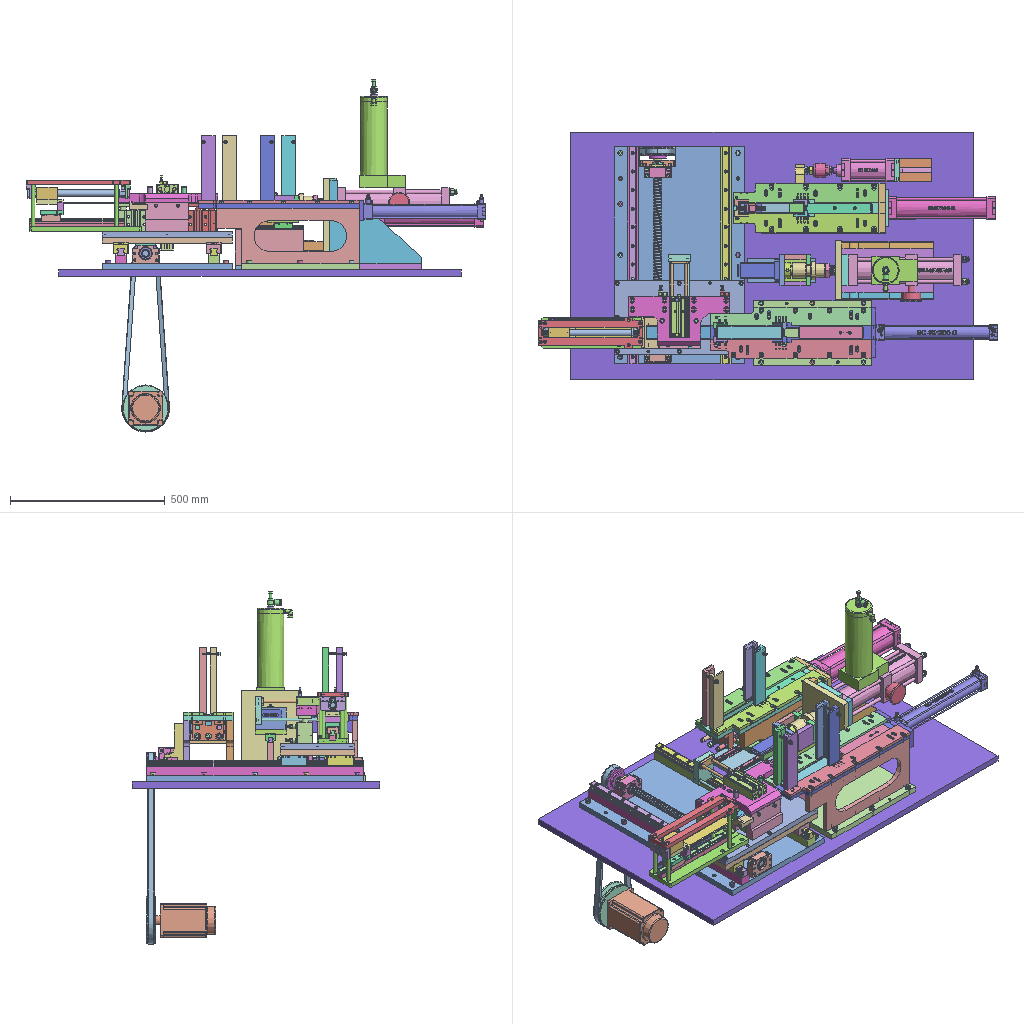Assembly | STEP file | 457 different items | 457 placed | box 1482 x 800 x 1137 mm
Parts list (item | name | quantity | parent item | size | volume), first 304 of 457 items:
1 | Tube feed_id1830_x_t | x1 | in Tube feed_x_t | 460 x 16 x 180 mm | 718962 mm3
2 | Tube feed_id1826_x_t | x1 | in Tube feed_x_t | 13.356 x 6 x 12 mm | 588.844 mm3
3 | Tube feed_id1822_x_t | x1 | in Tube feed_x_t | 13.356 x 6 x 12 mm | 588.844 mm3
4 | Tube feed_id1818_x_t | x1 | in Tube feed_x_t | 10 x 10 x 29.5 mm | 955.443 mm3
5 | Tube feed_id1814_x_t | x1 | in Tube feed_x_t | 10 x 10 x 29.5 mm | 955.443 mm3
6 | Tube feed_id1810_x_t | x1 | in Tube feed_x_t | 10 x 10 x 24.5 mm | 797.459 mm3
7 | Tube feed_id1806_x_t | x1 | in Tube feed_x_t | 10 x 10 x 24.5 mm | 797.459 mm3
8 | Tube feed_id1802_x_t | x1 | in Tube feed_x_t | 10 x 10 x 24.5 mm | 797.459 mm3
9 | Tube feed_id1798_x_t | x1 | in Tube feed_x_t | 10 x 10 x 24.5 mm | 797.459 mm3
10 | Tube feed_id1794_x_t | x1 | in Tube feed_x_t | 10 x 10 x 24.5 mm | 797.459 mm3
11 | Tube feed_id1790_x_t | x1 | in Tube feed_x_t | 8 x 22 x 23.5 mm | 3770 mm3
12 | Tube feed_id1786_x_t | x1 | in Tube feed_x_t | 8 x 22 x 23.5 mm | 3770 mm3
13 | Tube feed_id1782_x_t | x1 | in Tube feed_x_t | 8 x 22 x 23.5 mm | 3770 mm3
14 | Tube feed_id1778_x_t | x1 | in Tube feed_x_t | 8 x 22 x 23.5 mm | 3770 mm3
15 | Tube feed_id1774_x_t | x1 | in Tube feed_x_t | 520 x 160 x 13.5 mm | 851655 mm3
16 | Tube feed_id1770_x_t | x1 | in Tube feed_x_t | 380 x 208.2 x 19.5 mm | 1510900 mm3
17 | Tube feed_id1766_x_t | x1 | in Tube feed_x_t | 380 x 16 x 180 mm | 635735 mm3
18 | Tube feed_id1762_x_t | x1 | in Tube feed_x_t | 8 x 8 x 30 mm | 1469 mm3
19 | Tube feed_id1758_x_t | x1 | in Tube feed_x_t | 8 x 8 x 30 mm | 1469 mm3
20 | Tube feed_id1754_x_t | x1 | in Tube feed_x_t | 8 x 8 x 30 mm | 1469 mm3
21 | Tube feed_id1750_x_t | x1 | in Tube feed_x_t | 8 x 8 x 30 mm | 1469 mm3
22 | Tube feed_id1746_x_t | x1 | in Tube feed_x_t | 10 x 10 x 24.5 mm | 797.459 mm3
23 | Tube feed_id1742_x_t | x1 | in Tube feed_x_t | 13 x 13 x 33 mm | 1945 mm3
24 | Tube feed_id1738_x_t | x1 | in Tube feed_x_t | 8 x 8 x 40 mm | 1972 mm3
25 | Tube feed_id1734_x_t | x1 | in Tube feed_x_t | 8 x 8 x 40 mm | 1972 mm3
26 | Tube feed_id1730_x_t | x1 | in Tube feed_x_t | 16 x 16 x 50 mm | 4036 mm3
27 | Tube feed_id1726_x_t | x1 | in Tube feed_x_t | 16 x 16 x 50 mm | 4036 mm3
28 | Tube feed_id1722_x_t | x1 | in Tube feed_x_t | 16 x 16 x 50 mm | 4036 mm3
29 | Tube feed_id1718_x_t | x1 | in Tube feed_x_t | 16 x 16 x 50 mm | 4397 mm3
30 | Tube feed_id1714_x_t | x1 | in Tube feed_x_t | 16 x 16 x 50 mm | 4397 mm3
31 | Tube feed_id1710_x_t | x1 | in Tube feed_x_t | 16 x 16 x 50 mm | 4397 mm3
32 | Tube feed_id1706_x_t | x1 | in Tube feed_x_t | 8 x 8 x 35 mm | 1721 mm3
33 | Tube feed_id1702_x_t | x1 | in Tube feed_x_t | 8 x 8 x 35 mm | 1721 mm3
34 | Tube feed_id1698_x_t | x1 | in Tube feed_x_t | 8 x 8 x 35 mm | 1721 mm3
35 | Tube feed_id1694_x_t | x1 | in Tube feed_x_t | 8 x 8 x 35 mm | 1721 mm3
36 | Tube feed_id1690_x_t | x1 | in Tube feed_x_t | 13 x 13 x 33 mm | 1974 mm3
37 | Tube feed_id1686_x_t | x1 | in Tube feed_x_t | 13 x 13 x 33 mm | 1974 mm3
38 | Tube feed_id1682_x_t | x1 | in Tube feed_x_t | 13 x 13 x 33 mm | 1974 mm3
39 | Tube feed_id1678_x_t | x1 | in Tube feed_x_t | 13 x 13 x 33 mm | 1974 mm3
40 | Tube feed_id1674_x_t | x1 | in Tube feed_x_t | 13 x 13 x 33 mm | 1974 mm3
41 | Tube feed_id1670_x_t | x1 | in Tube feed_x_t | 13 x 13 x 33 mm | 1974 mm3
42 | Tube feed_id1666_x_t | x1 | in Tube feed_x_t | 13 x 13 x 33 mm | 1974 mm3
43 | Tube feed_id1662_x_t | x1 | in Tube feed_x_t | 13 x 13 x 33 mm | 1974 mm3
44 | Tube feed_id1658_x_t | x1 | in Tube feed_x_t | 13 x 13 x 33 mm | 1945 mm3
45 | Tube feed_id1654_x_t | x1 | in Tube feed_x_t | 13 x 13 x 33 mm | 1945 mm3
46 | Tube feed_id1650_x_t | x1 | in Tube feed_x_t | 13 x 13 x 33 mm | 1945 mm3
47 | Tube feed_id1646_x_t | x1 | in Tube feed_x_t | 13 x 13 x 33 mm | 1945 mm3
48 | Tube feed_id1642_x_t | x1 | in Tube feed_x_t | 13 x 13 x 33 mm | 1945 mm3
49 | Tube feed_id1638_x_t | x1 | in Tube feed_x_t | 13 x 13 x 33 mm | 1945 mm3
50 | Tube feed_id1634_x_t | x1 | in Tube feed_x_t | 13 x 13 x 33 mm | 1945 mm3
51 | Tube feed_id1630_x_t | x1 | in Tube feed_x_t | 13 x 13 x 33 mm | 1945 mm3
52 | Tube feed_id1626_x_t | x1 | in Tube feed_x_t | 16 x 16 x 47 mm | 3975 mm3
53 | Tube feed_id1622_x_t | x1 | in Tube feed_x_t | 16 x 16 x 47 mm | 3975 mm3
54 | Tube feed_id1618_x_t | x1 | in Tube feed_x_t | 16 x 16 x 47 mm | 3975 mm3
55 | Tube feed_id1614_x_t | x1 | in Tube feed_x_t | 16 x 16 x 47 mm | 3975 mm3
56 | Tube feed_id1610_x_t | x1 | in Tube feed_x_t | 16 x 16 x 47 mm | 3975 mm3
57 | Tube feed_id1606_x_t | x1 | in Tube feed_x_t | 10 x 10 x 26 mm | 858.061 mm3
58 | Tube feed_id1602_x_t | x1 | in Tube feed_x_t | 10 x 10 x 26 mm | 858.061 mm3
59 | Tube feed_id1598_x_t | x1 | in Tube feed_x_t | 10 x 10 x 26 mm | 858.061 mm3
60 | Tube feed_id1594_x_t | x1 | in Tube feed_x_t | 10 x 10 x 26 mm | 858.061 mm3
61 | Tube feed_id1590_x_t | x1 | in Tube feed_x_t | 10 x 10 x 26 mm | 858.061 mm3
62 | Tube feed_id1586_x_t | x1 | in Tube feed_x_t | 10 x 10 x 26 mm | 858.061 mm3
63 | Tube feed_id1582_x_t | x1 | in Tube feed_x_t | 10 x 10 x 26 mm | 858.061 mm3
64 | Tube feed_id1578_x_t | x1 | in Tube feed_x_t | 10 x 10 x 26 mm | 858.061 mm3
65 | Tube feed_id1574_x_t | x1 | in Tube feed_x_t | 10 x 10 x 26 mm | 858.061 mm3
66 | Tube feed_id1570_x_t | x1 | in Tube feed_x_t | 23 x 700 x 22 mm | 297908 mm3
67 | Tube feed_id1566_x_t | x1 | in Tube feed_x_t | 12 x 12 x 37 mm | 4054 mm3
68 | Tube feed_id1562_x_t | x1 | in Tube feed_x_t | 12 x 12 x 37 mm | 4054 mm3
69 | Tube feed_id1558_x_t | x1 | in Tube feed_x_t | 12 x 12 x 37 mm | 4054 mm3
70 | Tube feed_id1554_x_t | x1 | in Tube feed_x_t | 12 x 12 x 37 mm | 4054 mm3
71 | Tube feed_id1550_x_t | x1 | in Tube feed_x_t | 16 x 16 x 47 mm | 4055 mm3
72 | Tube feed_id1546_x_t | x1 | in Tube feed_x_t | 16 x 16 x 47 mm | 4055 mm3
73 | Tube feed_id1542_x_t | x1 | in Tube feed_x_t | 16 x 16 x 47 mm | 4055 mm3
74 | Tube feed_id1538_x_t | x1 | in Tube feed_x_t | 16 x 16 x 47 mm | 4055 mm3
75 | Tube feed_id1534_x_t | x1 | in Tube feed_x_t | 16 x 16 x 47 mm | 4055 mm3
76 | Tube feed_id1530_x_t | x1 | in Tube feed_x_t | 10 x 10 x 26 mm | 852.808 mm3
77 | Tube feed_id1526_x_t | x1 | in Tube feed_x_t | 10 x 10 x 26 mm | 852.808 mm3
78 | Tube feed_id1522_x_t | x1 | in Tube feed_x_t | 10 x 10 x 26 mm | 852.808 mm3
79 | Tube feed_id1518_x_t | x1 | in Tube feed_x_t | 10 x 10 x 26 mm | 852.808 mm3
80 | Tube feed_id1514_x_t | x1 | in Tube feed_x_t | 10 x 10 x 26 mm | 852.808 mm3
81 | Tube feed_id1510_x_t | x1 | in Tube feed_x_t | 10 x 10 x 26 mm | 852.808 mm3
82 | Tube feed_id1506_x_t | x1 | in Tube feed_x_t | 10 x 10 x 26 mm | 852.808 mm3
83 | Tube feed_id1502_x_t | x1 | in Tube feed_x_t | 10 x 10 x 26 mm | 852.808 mm3
84 | Tube feed_id1498_x_t | x1 | in Tube feed_x_t | 10 x 10 x 26 mm | 852.808 mm3
85 | Tube feed_id1494_x_t | x1 | in Tube feed_x_t | 10 x 10 x 26 mm | 852.808 mm3
86 | Tube feed_id1490_x_t | x1 | in Tube feed_x_t | 10 x 10 x 26 mm | 852.808 mm3
87 | Tube feed_id1486_x_t | x1 | in Tube feed_x_t | 10 x 10 x 26 mm | 852.808 mm3
88 | Tube feed_id1482_x_t | x1 | in Tube feed_x_t | 23 x 700 x 22 mm | 297908 mm3
89 | Tube feed_id1478_x_t | x1 | in Tube feed_x_t | 10 x 10 x 26 mm | 858.061 mm3
90 | Tube feed_id1474_x_t | x1 | in Tube feed_x_t | 10 x 10 x 26 mm | 858.061 mm3
91 | Tube feed_id1470_x_t | x1 | in Tube feed_x_t | 10 x 10 x 26 mm | 858.061 mm3
92 | Tube feed_id1466_x_t | x1 | in Tube feed_x_t | 35 x 700 x 30 mm | 688178 mm3
93 | Tube feed_id1462_x_t | x1 | in Tube feed_x_t | 35 x 700 x 30 mm | 688178 mm3
94 | Tube feed_id1458_x_t | x1 | in Tube feed_x_t | 13 x 13 x 28 mm | 1716 mm3
95 | Tube feed_id1454_x_t | x1 | in Tube feed_x_t | 13 x 13 x 28 mm | 1716 mm3
96 | Tube feed_id1450_x_t | x1 | in Tube feed_x_t | 13 x 13 x 28 mm | 1716 mm3
97 | Tube feed_id1446_x_t | x1 | in Tube feed_x_t | 13 x 13 x 28 mm | 1716 mm3
98 | Tube feed_id1442_x_t | x1 | in Tube feed_x_t | 13 x 13 x 28 mm | 1716 mm3
99 | Tube feed_id1438_x_t | x1 | in Tube feed_x_t | 13 x 13 x 28 mm | 1716 mm3
100 | Tube feed_id1434_x_t | x1 | in Tube feed_x_t | 13 x 13 x 28 mm | 1716 mm3
101 | Tube feed_id1430_x_t | x1 | in Tube feed_x_t | 13 x 13 x 28 mm | 1716 mm3
102 | Tube feed_id1426_x_t | x1 | in Tube feed_x_t | 13 x 13 x 28 mm | 1716 mm3
103 | Tube feed_id1422_x_t | x1 | in Tube feed_x_t | 13 x 13 x 28 mm | 1716 mm3
104 | Tube feed_id1418_x_t | x1 | in Tube feed_x_t | 13 x 13 x 28 mm | 1716 mm3
105 | Tube feed_id1414_x_t | x1 | in Tube feed_x_t | 13 x 13 x 28 mm | 1716 mm3
106 | Tube feed_id1410_x_t | x1 | in Tube feed_x_t | 8 x 8 x 30 mm | 1469 mm3
107 | Tube feed_id1406_x_t | x1 | in Tube feed_x_t | 8 x 8 x 30 mm | 1469 mm3
108 | Tube feed_id1402_x_t | x1 | in Tube feed_x_t | 8 x 8 x 30 mm | 1469 mm3
109 | Tube feed_id1398_x_t | x1 | in Tube feed_x_t | 8 x 8 x 30 mm | 1469 mm3
110 | Tube feed_id1394_x_t | x1 | in Tube feed_x_t | 8 x 8 x 30 mm | 1469 mm3
111 | Tube feed_id1390_x_t | x1 | in Tube feed_x_t | 8 x 8 x 30 mm | 1469 mm3
112 | 25 lead screw BK_id1386_x_t | x1 | in Tube feed_x_t | 25 x 669.5 x 25 mm | 331480 mm3
113 | BF-20_id1382_x_t | x1 | in Tube feed_x_t | 42 x 12 x 42 mm | 3541 mm3
114 | BF-20_id1378_x_t | x1 | in Tube feed_x_t | 7 x 7 x 7 mm | 179.594 mm3
115 | BF-20_id1374_x_t | x1 | in Tube feed_x_t | - | 179.594 mm3
116 | BF-20_id1370_x_t | x1 | in Tube feed_x_t | - | 179.594 mm3
117 | BF-20_id1366_x_t | x1 | in Tube feed_x_t | 25 x 12 x 25 mm | 2005 mm3
118 | BF-20_id1362_x_t | x1 | in Tube feed_x_t | - | 179.594 mm3
119 | BF-20_id1358_x_t | x1 | in Tube feed_x_t | 7 x 7 x 7 mm | 179.594 mm3
120 | BF-20_id1354_x_t | x1 | in Tube feed_x_t | - | 179.594 mm3
121 | BF-20_id1350_x_t | x1 | in Tube feed_x_t | - | 179.594 mm3
122 | BF-20_id1346_x_t | x1 | in Tube feed_x_t | - | 179.594 mm3
123 | BF-20_id1342_x_t | x1 | in Tube feed_x_t | - | 179.594 mm3
124 | BF-20_id1338_x_t | x1 | in Tube feed_x_t | 88 x 26 x 60 mm | 81051 mm3
125 | BF-20_id1334_x_t | x1 | in Tube feed_x_t | - | 179.594 mm3
126 | BF-20_id1330_x_t | x1 | in Tube feed_x_t | - | 179.594 mm3
127 | BF-20_id1326_x_t | x1 | in Tube feed_x_t | - | 179.594 mm3
128 | BF-20_id1322_x_t | x1 | in Tube feed_x_t | - | 179.594 mm3
129 | BF-20_id1318_x_t | x1 | in Tube feed_x_t | - | 179.594 mm3
130 | BK-20_id1314_x_t | x1 | in Tube feed_x_t | 42 x 12 x 42 mm | 3939 mm3
131 | BK-20_id1310_x_t | x1 | in Tube feed_x_t | 42 x 12 x 42 mm | 4062 mm3
132 | BK-20_id1306_x_t | x1 | in Tube feed_x_t | 6.35 x 6.35 x 6.35 mm | 134.066 mm3
133 | BK-20_id1302_x_t | x1 | in Tube feed_x_t | 6.35 x 6.35 x 6.35 mm | 134.066 mm3
134 | BK-20_id1298_x_t | x1 | in Tube feed_x_t | 6.35 x 6.35 x 6.35 mm | 134.066 mm3
135 | BK-20_id1294_x_t | x1 | in Tube feed_x_t | 6.35 x 6.35 x 6.35 mm | 134.066 mm3
136 | BK-20_id1290_x_t | x1 | in Tube feed_x_t | 6.35 x 6.35 x 6.35 mm | 134.066 mm3
137 | BK-20_id1286_x_t | x1 | in Tube feed_x_t | 6.35 x 6.35 x 6.35 mm | 134.066 mm3
138 | BK-20_id1282_x_t | x1 | in Tube feed_x_t | 6.35 x 6.35 x 6.35 mm | 134.066 mm3
139 | BK-20_id1278_x_t | x1 | in Tube feed_x_t | 6.35 x 6.35 x 6.35 mm | 134.066 mm3
140 | BK-20_id1274_x_t | x1 | in Tube feed_x_t | 6.35 x 6.35 x 6.35 mm | 134.066 mm3
141 | BK-20_id1270_x_t | x1 | in Tube feed_x_t | 6.35 x 6.35 x 6.35 mm | 134.066 mm3
142 | BK-20_id1266_x_t | x1 | in Tube feed_x_t | 6.35 x 6.35 x 6.35 mm | 134.066 mm3
143 | BK-20_id1262_x_t | x1 | in Tube feed_x_t | 6.35 x 6.35 x 6.35 mm | 134.066 mm3
144 | BK-20_id1258_x_t | x1 | in Tube feed_x_t | 6.35 x 6.35 x 6.35 mm | 134.066 mm3
145 | BK-20_id1254_x_t | x1 | in Tube feed_x_t | 27.5 x 12 x 27.5 mm | 2449 mm3
146 | BK-20_id1250_x_t | x1 | in Tube feed_x_t | 27.5 x 12 x 27.5 mm | 2436 mm3
147 | BK-20_id1246_x_t | x1 | in Tube feed_x_t | 25.4 x 8 x 25.4 mm | 1515 mm3
148 | BK-20_id1242_x_t | x1 | in Tube feed_x_t | 6.35 x 6.35 x 6.35 mm | 134.066 mm3
149 | BK-20_id1238_x_t | x1 | in Tube feed_x_t | 6.35 x 6.35 x 6.35 mm | 134.066 mm3
150 | BK-20_id1234_x_t | x1 | in Tube feed_x_t | 38 x 6 x 38 mm | 1518 mm3
151 | BK-20_id1230_x_t | x1 | in Tube feed_x_t | 6.35 x 6.35 x 6.35 mm | 134.066 mm3
152 | BK-20_id1226_x_t | x1 | in Tube feed_x_t | 38 x 6 x 38 mm | 1557 mm3
153 | BK-20_id1222_x_t | x1 | in Tube feed_x_t | 6.35 x 6.35 x 6.35 mm | 134.066 mm3
154 | BK-20_id1218_x_t | x1 | in Tube feed_x_t | 6.35 x 6.35 x 6.35 mm | 134.066 mm3
155 | BK-20_id1214_x_t | x1 | in Tube feed_x_t | 50 x 11.15 x 50 mm | 9475 mm3
156 | BK-20_id1210_x_t | x1 | in Tube feed_x_t | 6.35 x 6.35 x 6.35 mm | 134.066 mm3
157 | BK-20_id1206_x_t | x1 | in Tube feed_x_t | 35 x 11 x 35 mm | 5569 mm3
158 | BK-20_id1202_x_t | x1 | in Tube feed_x_t | 6.35 x 6.35 x 6.35 mm | 134.066 mm3
159 | BK-20_id1198_x_t | x1 | in Tube feed_x_t | 6.35 x 6.35 x 6.35 mm | 134.066 mm3
160 | BK-20_id1194_x_t | x1 | in Tube feed_x_t | 6.35 x 6.35 x 6.35 mm | 134.066 mm3
161 | BK-20_id1190_x_t | x1 | in Tube feed_x_t | 88 x 35 x 60 mm | 106061 mm3
162 | BK-20_id1186_x_t | x1 | in Tube feed_x_t | 6.35 x 6.35 x 6.35 mm | 134.066 mm3
163 | BK-20_id1182_x_t | x1 | in Tube feed_x_t | 6.35 x 6.35 x 6.35 mm | 134.066 mm3
164 | BK-20_id1178_x_t | x1 | in Tube feed_x_t | 6.35 x 6.35 x 6.35 mm | 134.066 mm3
165 | BK-20_id1174_x_t | x1 | in Tube feed_x_t | 6.35 x 6.35 x 6.35 mm | 134.066 mm3
166 | BK-20_id1170_x_t | x1 | in Tube feed_x_t | 25.4 x 8.5 x 25.4 mm | 1588 mm3
167 | Tube feed_id1166_x_t | x1 | in Tube feed_x_t | 420 x 700 x 19.5 mm | 5525930 mm3
168 | Tube feed_id1162_x_t | x1 | in Tube feed_x_t | 13 x 13 x 68 mm | 3686 mm3
169 | Tube feed_id1158_x_t | x1 | in Tube feed_x_t | 13 x 13 x 68 mm | 3686 mm3
170 | Tube feed_id1154_x_t | x1 | in Tube feed_x_t | 13 x 13 x 68 mm | 3686 mm3
171 | Tube feed_id1150_x_t | x1 | in Tube feed_x_t | 13 x 13 x 68 mm | 3686 mm3
172 | Tube feed_id1146_x_t | x1 | in Tube feed_x_t | 13 x 13 x 68 mm | 3686 mm3
173 | Tube feed_id1142_x_t | x1 | in Tube feed_x_t | 13 x 13 x 68 mm | 3686 mm3
174 | Tube feed_id1138_x_t | x1 | in Tube feed_x_t | 8 x 8 x 20 mm | 966.7 mm3
175 | Tube feed_id1134_x_t | x1 | in Tube feed_x_t | 8 x 8 x 20 mm | 966.7 mm3
176 | Tube feed_id1130_x_t | x1 | in Tube feed_x_t | 13 x 13 x 33 mm | 1997 mm3
177 | Tube feed_id1126_x_t | x1 | in Tube feed_x_t | 13 x 13 x 33 mm | 1997 mm3
178 | Tube feed_id1122_x_t | x1 | in Tube feed_x_t | 13 x 13 x 33 mm | 1997 mm3
179 | Tube feed_id1118_x_t | x1 | in Tube feed_x_t | 13 x 13 x 33 mm | 1997 mm3
180 | Tube feed_id1114_x_t | x1 | in Tube feed_x_t | 13 x 13 x 33 mm | 1997 mm3
181 | Tube feed_id1110_x_t | x1 | in Tube feed_x_t | 13 x 13 x 33 mm | 1997 mm3
182 | Tube feed_id1106_x_t | x1 | in Tube feed_x_t | 13 x 13 x 33 mm | 1997 mm3
183 | Tube feed_id1102_x_t | x1 | in Tube feed_x_t | 13 x 13 x 33 mm | 1997 mm3
184 | Tube feed_id1098_x_t | x1 | in Tube feed_x_t | 10 x 10 x 21 mm | 739.091 mm3
185 | Tube feed_id1094_x_t | x1 | in Tube feed_x_t | 10 x 10 x 21 mm | 739.091 mm3
186 | Tube feed_id1090_x_t | x1 | in Tube feed_x_t | 10 x 10 x 21 mm | 739.091 mm3
187 | Tube feed_id1086_x_t | x1 | in Tube feed_x_t | 10 x 10 x 21 mm | 739.091 mm3
188 | Tube feed_id1082_x_t | x1 | in Tube feed_x_t | 10 x 10 x 21 mm | 739.091 mm3
189 | Tube feed_id1078_x_t | x1 | in Tube feed_x_t | 10 x 10 x 21 mm | 739.091 mm3
190 | Tube feed_id1074_x_t | x1 | in Tube feed_x_t | 10 x 10 x 21 mm | 739.091 mm3
191 | Tube feed_id1070_x_t | x1 | in Tube feed_x_t | 10 x 10 x 21 mm | 739.091 mm3
192 | Tube feed_id1066_x_t | x1 | in Tube feed_x_t | 10 x 10 x 21 mm | 739.091 mm3
193 | Tube feed_id1062_x_t | x1 | in Tube feed_x_t | 10 x 10 x 21 mm | 739.091 mm3
194 | Tube feed_id1058_x_t | x1 | in Tube feed_x_t | 10 x 10 x 21 mm | 739.091 mm3
195 | Tube feed_id1054_x_t | x1 | in Tube feed_x_t | 10 x 10 x 21 mm | 739.091 mm3
196 | Tube feed_id1050_x_t | x1 | in Tube feed_x_t | 10 x 10 x 21 mm | 739.091 mm3
197 | Tube feed_id1046_x_t | x1 | in Tube feed_x_t | 10 x 10 x 21 mm | 739.091 mm3
198 | Tube feed_id1042_x_t | x1 | in Tube feed_x_t | 10 x 10 x 21 mm | 739.091 mm3
199 | Tube feed_id1038_x_t | x1 | in Tube feed_x_t | 10 x 10 x 21 mm | 739.091 mm3
200 | Tube feed_id1034_x_t | x1 | in Tube feed_x_t | 10 x 10 x 41 mm | 1187 mm3
201 | Tube feed_id1030_x_t | x1 | in Tube feed_x_t | 10 x 10 x 41 mm | 1187 mm3
202 | Tube feed_id1026_x_t | x1 | in Tube feed_x_t | 10 x 10 x 41 mm | 1187 mm3
203 | Tube feed_id1022_x_t | x1 | in Tube feed_x_t | 10 x 10 x 41 mm | 1187 mm3
204 | Tube feed_id1018_x_t | x1 | in Tube feed_x_t | 66 x 40 x 8 mm | 19888 mm3
205 | Tube feed_id1014_x_t | x1 | in Tube feed_x_t | 420 x 240 x 19.3 mm | 1597092 mm3
206 | SFU2510 nut seat_id1010_x_t | x1 | in Tube feed_x_t | 66 x 85 x 48 mm | 143394 mm3
207 | Tube feed_id1006_x_t | x1 | in Tube feed_x_t | 48 x 95 x 34.5 mm | 104775 mm3
208 | Tube feed_id1002_x_t | x1 | in Tube feed_x_t | 48 x 95 x 34.5 mm | 104775 mm3
209 | Tube feed_id998_x_t | x1 | in Tube feed_x_t | 48 x 95 x 34.5 mm | 104775 mm3
210 | Tube feed_id994_x_t | x1 | in Tube feed_x_t | 48 x 95 x 34.5 mm | 104775 mm3
211 | Tube feed_id990_x_t | x1 | in Tube feed_x_t | 10 x 56 x 10 mm | 1498 mm3
212 | Tube feed_id986_x_t | x1 | in Tube feed_x_t | 10 x 56 x 10 mm | 1498 mm3
213 | Tube feed_id982_x_t | x1 | in Tube feed_x_t | 8 x 19.5 x 8 mm | 422.965 mm3
214 | Tube feed_id978_x_t | x1 | in Tube feed_x_t | 8 x 19.5 x 8 mm | 422.965 mm3
215 | Tube feed_id974_x_t | x1 | in Tube feed_x_t | 8 x 19.5 x 8 mm | 422.965 mm3
216 | Tube feed_id970_x_t | x1 | in Tube feed_x_t | 8 x 19.5 x 8 mm | 422.965 mm3
217 | Tube feed_id966_x_t | x1 | in Tube feed_x_t | 8 x 19.5 x 8 mm | 422.965 mm3
218 | Tube feed_id962_x_t | x1 | in Tube feed_x_t | 8 x 19.5 x 8 mm | 429.516 mm3
219 | Tube feed_id958_x_t | x1 | in Tube feed_x_t | 8 x 19.5 x 8 mm | 429.516 mm3
220 | Tube feed_id954_x_t | x1 | in Tube feed_x_t | 520 x 59.75 x 11 mm | 276450 mm3
221 | Tube feed_id950_x_t | x1 | in Tube feed_x_t | 520 x 59.75 x 11 mm | 287965 mm3
222 | Tube feed_id946_x_t | x1 | in Tube feed_x_t | 15 x 15 x 22 mm | 3354 mm3
223 | Tube feed_id942_x_t | x1 | in Tube feed_x_t | 40.4 x 59.9 x 46.8 mm | 59964 mm3
224 | Tube feed_id938_x_t | x1 | in Tube feed_x_t | 8 x 8 x 67 mm | 3084 mm3
225 | Tube feed_id934_x_t | x1 | in Tube feed_x_t | 8 x 8 x 67 mm | 3084 mm3
226 | Tube feed_id930_x_t | x1 | in Tube feed_x_t | 8 x 8 x 67 mm | 3084 mm3
227 | Tube feed_id926_x_t | x1 | in Tube feed_x_t | 8 x 8 x 67 mm | 3084 mm3
228 | Tube feed_id922_x_t | x1 | in Tube feed_x_t | 125 x 45 x 25 mm | 129874 mm3
229 | Tube feed_id918_x_t | x1 | in Tube feed_x_t | 140 x 100 x 94 mm | 657707 mm3
230 | Tube feed_id914_x_t | x1 | in Tube feed_x_t | 205 x 45.1 x 5.7 mm | 9751 mm3
231 | Tube feed_id910_x_t | x1 | in Tube feed_x_t | 244.5 x 43.6 x 4.2 mm | 43290 mm3
232 | Tube feed_id906_x_t | x1 | in Tube feed_x_t | 15 x 15 x 105 mm | 18472 mm3
233 | Tube feed_id902_x_t | x1 | in Tube feed_x_t | 15 x 15 x 105 mm | 18472 mm3
234 | Tube feed_id898_x_t | x1 | in Tube feed_x_t | 122.75 x 88 x 116 mm | 476709 mm3
235 | Tube feed_id894_x_t | x1 | in Tube feed_x_t | 420 x 240 x 19.3 mm | 1848143 mm3
236 | Tube feed_id890_x_t | x1 | in Tube feed_x_t | 64 x 137.8 x 30 mm | 193206 mm3
237 | Tube feed_id886_x_t | x1 | in Tube feed_x_t | 325 x 161 x 30 mm | 914325 mm3
238 | Tube feed_id882_x_t | x1 | in Tube feed_x_t | 70 x 203.3 x 90 mm | 152546 mm3
239 | Tube feed_id878_x_t | x1 | in Tube feed_x_t | 62 x 165.8 x 25 mm | 36735 mm3
240 | Tube feed_id874_x_t | x1 | in Tube feed_x_t | 1300 x 800 x 21 mm | 21652093 mm3
241 | Tube feed_id870_x_t | x1 | in Tube feed_x_t | 305 x 14.464 x 15 mm | 56339 mm3
242 | Tube feed_id866_x_t | x1 | in Tube feed_x_t | 305 x 20 x 20 mm | 102341 mm3
243 | Tube feed_id862_x_t | x1 | in Tube feed_x_t | 205 x 45.1 x 5.7 mm | 9751 mm3
244 | Tube feed_id858_x_t | x1 | in Tube feed_x_t | 86 x 65 x 14.5 mm | 52880 mm3
245 | Tube feed_id854_x_t | x1 | in Tube feed_x_t | 20 x 65 x 26.1 mm | 28245 mm3
246 | Tube feed_id850_x_t | x1 | in Tube feed_x_t | 73 x 65 x 14 mm | 44658 mm3
247 | Tube feed_id846_x_t | x1 | in Tube feed_x_t | 61.4 x 34 x 23.7 mm | 39681 mm3
248 | Tube feed_id842_x_t | x1 | in Tube feed_x_t | 252 x 13 x 10 mm | 22066 mm3
249 | Tube feed_id838_x_t | x1 | in Tube feed_x_t | 360 x 100 x 155 mm | 559892 mm3
250 | Tube feed_id834_x_t | x1 | in Tube feed_x_t | 6 x 27 x 30.677 mm | 2131 mm3
251 | Tube feed_id830_x_t | x1 | in Tube feed_x_t | 6 x 27 x 30.677 mm | 2131 mm3
252 | Tube feed_id826_x_t | x1 | in Tube feed_x_t | 66 x 45 x 40 mm | 90173 mm3
253 | Tube feed_id822_x_t | x1 | in Tube feed_x_t | 15 x 80 x 45 mm | 22144 mm3
254 | Tube feed_id818_x_t | x1 | in Tube feed_x_t | 15 x 80 x 45 mm | 22144 mm3
255 | Tube feed_id814_x_t | x1 | in Tube feed_x_t | 336 x 100 x 15 mm | 239179 mm3
256 | Tube feed_id810_x_t | x1 | in Tube feed_x_t | 330 x 33.15 x 53.75 mm | 129080 mm3
257 | Tube feed_id806_x_t | x1 | in Tube feed_x_t | 13.856 x 12 x 4 mm | 488.727 mm3
258 | Tube feed_id802_x_t | x1 | in Tube feed_x_t | 7 x 7 x 7 mm | 153.655 mm3
259 | Tube feed_id798_x_t | x1 | in Tube feed_x_t | 10 x 21.824 x 18.9 mm | 3030 mm3
260 | Tube feed_id794_x_t | x1 | in Tube feed_x_t | 344 x 16 x 16 mm | 68432 mm3
261 | Tube feed_id790_x_t | x1 | in Tube feed_x_t | 15 x 160 x 65 mm | 131151 mm3
262 | Tube feed_id786_x_t | x1 | in Tube feed_x_t | 40 x 45 x 40 mm | 56393 mm3
263 | Tube feed_id782_x_t | x1 | in Tube feed_x_t | 210 x 40 x 5 mm | 41286 mm3
264 | Tube feed_id778_x_t | x1 | in Tube feed_x_t | 295 x 20 x 270 mm | 766863 mm3
265 | Tube feed_id774_x_t | x1 | in Tube feed_x_t | 20 x 190 x 295 mm | 1060619 mm3
266 | Tube feed_id770_x_t | x1 | in Tube feed_x_t | 295 x 190 x 20 mm | 1121000 mm3
267 | Tube feed_id766_x_t | x1 | in Tube feed_x_t | 7 x 7 x 7 mm | 153.655 mm3
268 | Tube feed_id762_x_t | x1 | in Tube feed_x_t | 13.856 x 12 x 4 mm | 488.727 mm3
269 | Tube feed_id758_x_t | x1 | in Tube feed_x_t | 10 x 21.824 x 18.9 mm | 3030 mm3
270 | Tube feed_id754_x_t | x1 | in Tube feed_x_t | - | -
271 | Tube feed_id750_x_t | x1 | in Tube feed_x_t | 146 x 116.5 x 295 mm | 2001798 mm3
272 | Tube feed_id746_x_t | x1 | in Tube feed_x_t | 435 x 100 x 100 mm | 2482433 mm3
273 | Tube feed_id742_x_t | x1 | in Tube feed_x_t | 20 x 100 x 160 mm | 294867 mm3
274 | Tube feed_id738_x_t | x1 | in Tube feed_x_t | 295 x 20 x 270 mm | 766863 mm3
275 | Tube feed_id734_x_t | x1 | in Tube feed_x_t | 24.249 x 21 x 7 mm | 1738 mm3
276 | Tube feed_id730_x_t | x1 | in Tube feed_x_t | 22 x 45.08 x 53 mm | 14856 mm3
277 | Tube feed_id726_x_t | x1 | in Tube feed_x_t | 70 x 50 x 70 mm | 100586 mm3
278 | Tube feed_id722_x_t | x1 | in Tube feed_x_t | 6 x 18 x 20.785 mm | 1113 mm3
279 | Tube feed_id718_x_t | x1 | in Tube feed_x_t | 22 x 18 x 20.785 mm | 3414 mm3
280 | Tube feed_id714_x_t | x1 | in Tube feed_x_t | 6 x 18 x 20.785 mm | 1113 mm3
281 | Tube feed_id710_x_t | x1 | in Tube feed_x_t | 22 x 18 x 20.785 mm | 3414 mm3
282 | Tube feed_id706_x_t | x1 | in Tube feed_x_t | 6 x 18 x 20.785 mm | 1113 mm3
283 | Tube feed_id702_x_t | x1 | in Tube feed_x_t | 22 x 18 x 20.785 mm | 3414 mm3
284 | Tube feed_id698_x_t | x1 | in Tube feed_x_t | 22 x 18 x 20.785 mm | 3414 mm3
285 | Tube feed_id694_x_t | x1 | in Tube feed_x_t | 15 x 46 x 53.116 mm | 17601 mm3
286 | Tube feed_id690_x_t | x1 | in Tube feed_x_t | 6 x 18 x 20.785 mm | 1113 mm3
287 | Tube feed_id686_x_t | x1 | in Tube feed_x_t | 106 x 60 x 60 mm | 191501 mm3
288 | Tube feed_id682_x_t | x1 | in Tube feed_x_t | 70 x 15 x 70 mm | 73500 mm3
289 | Tube feed_id678_x_t | x1 | in Tube feed_x_t | 15 x 100 x 70 mm | 81265 mm3
290 | Tube feed_id674_x_t | x1 | in Tube feed_x_t | 70 x 15 x 70 mm | 73500 mm3
291 | Tube feed_id670_x_t | x1 | in Tube feed_x_t | 15 x 100 x 70 mm | 105000 mm3
292 | Tube feed_id666_x_t | x1 | in Tube feed_x_t | 100 x 100 x 15 mm | 141686 mm3
293 | Tube feed_id662_x_t | x1 | in Tube feed_x_t | 57 x 30 x 30 mm | 35009 mm3
294 | Tube feed_id658_x_t | x1 | in Tube feed_x_t | 470 x 160 x 15 mm | 862310 mm3
295 | Tube feed_id654_x_t | x1 | in Tube feed_x_t | 380 x 20 x 137 mm | 613484 mm3
296 | Tube feed_id650_x_t | x1 | in Tube feed_x_t | 380 x 20 x 137 mm | 613484 mm3
297 | Tube feed_id646_x_t | x1 | in Tube feed_x_t | 290 x 160 x 20 mm | 842300 mm3
298 | Tube feed_id642_x_t | x1 | in Tube feed_x_t | 400 x 15 x 15 mm | 78237 mm3
299 | Tube feed_id638_x_t | x1 | in Tube feed_x_t | 400 x 160 x 20 mm | 1244000 mm3
300 | Tube feed_id634_x_t | x1 | in Tube feed_x_t | 7 x 7 x 19 mm | 320.116 mm3
301 | Tube feed_id630_x_t | x1 | in Tube feed_x_t | 7 x 7 x 19 mm | 320.116 mm3
302 | Tube feed_id626_x_t | x1 | in Tube feed_x_t | 7 x 7 x 19 mm | 320.116 mm3
303 | Tube feed_id622_x_t | x1 | in Tube feed_x_t | 7 x 7 x 19 mm | 320.116 mm3
304 | Tube feed_id618_x_t | x1 | in Tube feed_x_t | 137 x 70 x 36 mm | 107934 mm3
Placements (level | parent | child | x y z in mm | rotation matrix by rows), first 215 of 457 lines:
1 | Tube feed_x_t | Tube feed_id1830_x_t | 0.0 0.0 0.0 | 1 0 0 0 1 0 0 0 1
1 | Tube feed_x_t | Tube feed_id1826_x_t | 0.0 0.0 0.0 | 1 0 0 0 1 0 0 0 1
1 | Tube feed_x_t | Tube feed_id1822_x_t | 0.0 0.0 0.0 | 1 0 0 0 1 0 0 0 1
1 | Tube feed_x_t | Tube feed_id1818_x_t | 0.0 0.0 0.0 | 1 0 0 0 1 0 0 0 1
1 | Tube feed_x_t | Tube feed_id1814_x_t | 0.0 0.0 0.0 | 1 0 0 0 1 0 0 0 1
1 | Tube feed_x_t | Tube feed_id1810_x_t | 0.0 0.0 0.0 | 1 0 0 0 1 0 0 0 1
1 | Tube feed_x_t | Tube feed_id1806_x_t | 0.0 0.0 0.0 | 1 0 0 0 1 0 0 0 1
1 | Tube feed_x_t | Tube feed_id1802_x_t | 0.0 0.0 0.0 | 1 0 0 0 1 0 0 0 1
1 | Tube feed_x_t | Tube feed_id1798_x_t | 0.0 0.0 0.0 | 1 0 0 0 1 0 0 0 1
1 | Tube feed_x_t | Tube feed_id1794_x_t | 0.0 0.0 0.0 | 1 0 0 0 1 0 0 0 1
1 | Tube feed_x_t | Tube feed_id1790_x_t | 0.0 0.0 0.0 | 1 0 0 0 1 0 0 0 1
1 | Tube feed_x_t | Tube feed_id1786_x_t | 0.0 0.0 0.0 | 1 0 0 0 1 0 0 0 1
1 | Tube feed_x_t | Tube feed_id1782_x_t | 0.0 0.0 0.0 | 1 0 0 0 1 0 0 0 1
1 | Tube feed_x_t | Tube feed_id1778_x_t | 0.0 0.0 0.0 | 1 0 0 0 1 0 0 0 1
1 | Tube feed_x_t | Tube feed_id1774_x_t | 0.0 0.0 0.0 | 1 0 0 0 1 0 0 0 1
1 | Tube feed_x_t | Tube feed_id1770_x_t | 0.0 0.0 0.0 | 1 0 0 0 1 0 0 0 1
1 | Tube feed_x_t | Tube feed_id1766_x_t | 0.0 0.0 0.0 | 1 0 0 0 1 0 0 0 1
1 | Tube feed_x_t | Tube feed_id1762_x_t | 0.0 0.0 0.0 | 1 0 0 0 1 0 0 0 1
1 | Tube feed_x_t | Tube feed_id1758_x_t | 0.0 0.0 0.0 | 1 0 0 0 1 0 0 0 1
1 | Tube feed_x_t | Tube feed_id1754_x_t | 0.0 0.0 0.0 | 1 0 0 0 1 0 0 0 1
1 | Tube feed_x_t | Tube feed_id1750_x_t | 0.0 0.0 0.0 | 1 0 0 0 1 0 0 0 1
1 | Tube feed_x_t | Tube feed_id1746_x_t | 0.0 0.0 0.0 | 1 0 0 0 1 0 0 0 1
1 | Tube feed_x_t | Tube feed_id1742_x_t | 0.0 0.0 0.0 | 1 0 0 0 1 0 0 0 1
1 | Tube feed_x_t | Tube feed_id1738_x_t | 0.0 0.0 0.0 | 1 0 0 0 1 0 0 0 1
1 | Tube feed_x_t | Tube feed_id1734_x_t | 0.0 0.0 0.0 | 1 0 0 0 1 0 0 0 1
1 | Tube feed_x_t | Tube feed_id1730_x_t | 0.0 0.0 0.0 | 1 0 0 0 1 0 0 0 1
1 | Tube feed_x_t | Tube feed_id1726_x_t | 0.0 0.0 0.0 | 1 0 0 0 1 0 0 0 1
1 | Tube feed_x_t | Tube feed_id1722_x_t | 0.0 0.0 0.0 | 1 0 0 0 1 0 0 0 1
1 | Tube feed_x_t | Tube feed_id1718_x_t | 0.0 0.0 0.0 | 1 0 0 0 1 0 0 0 1
1 | Tube feed_x_t | Tube feed_id1714_x_t | 0.0 0.0 0.0 | 1 0 0 0 1 0 0 0 1
1 | Tube feed_x_t | Tube feed_id1710_x_t | 0.0 0.0 0.0 | 1 0 0 0 1 0 0 0 1
1 | Tube feed_x_t | Tube feed_id1706_x_t | 0.0 0.0 0.0 | 1 0 0 0 1 0 0 0 1
1 | Tube feed_x_t | Tube feed_id1702_x_t | 0.0 0.0 0.0 | 1 0 0 0 1 0 0 0 1
1 | Tube feed_x_t | Tube feed_id1698_x_t | 0.0 0.0 0.0 | 1 0 0 0 1 0 0 0 1
1 | Tube feed_x_t | Tube feed_id1694_x_t | 0.0 0.0 0.0 | 1 0 0 0 1 0 0 0 1
1 | Tube feed_x_t | Tube feed_id1690_x_t | 0.0 0.0 0.0 | 1 0 0 0 1 0 0 0 1
1 | Tube feed_x_t | Tube feed_id1686_x_t | 0.0 0.0 0.0 | 1 0 0 0 1 0 0 0 1
1 | Tube feed_x_t | Tube feed_id1682_x_t | 0.0 0.0 0.0 | 1 0 0 0 1 0 0 0 1
1 | Tube feed_x_t | Tube feed_id1678_x_t | 0.0 0.0 0.0 | 1 0 0 0 1 0 0 0 1
1 | Tube feed_x_t | Tube feed_id1674_x_t | 0.0 0.0 0.0 | 1 0 0 0 1 0 0 0 1
1 | Tube feed_x_t | Tube feed_id1670_x_t | 0.0 0.0 0.0 | 1 0 0 0 1 0 0 0 1
1 | Tube feed_x_t | Tube feed_id1666_x_t | 0.0 0.0 0.0 | 1 0 0 0 1 0 0 0 1
1 | Tube feed_x_t | Tube feed_id1662_x_t | 0.0 0.0 0.0 | 1 0 0 0 1 0 0 0 1
1 | Tube feed_x_t | Tube feed_id1658_x_t | 0.0 0.0 0.0 | 1 0 0 0 1 0 0 0 1
1 | Tube feed_x_t | Tube feed_id1654_x_t | 0.0 0.0 0.0 | 1 0 0 0 1 0 0 0 1
1 | Tube feed_x_t | Tube feed_id1650_x_t | 0.0 0.0 0.0 | 1 0 0 0 1 0 0 0 1
1 | Tube feed_x_t | Tube feed_id1646_x_t | 0.0 0.0 0.0 | 1 0 0 0 1 0 0 0 1
1 | Tube feed_x_t | Tube feed_id1642_x_t | 0.0 0.0 0.0 | 1 0 0 0 1 0 0 0 1
1 | Tube feed_x_t | Tube feed_id1638_x_t | 0.0 0.0 0.0 | 1 0 0 0 1 0 0 0 1
1 | Tube feed_x_t | Tube feed_id1634_x_t | 0.0 0.0 0.0 | 1 0 0 0 1 0 0 0 1
1 | Tube feed_x_t | Tube feed_id1630_x_t | 0.0 0.0 0.0 | 1 0 0 0 1 0 0 0 1
1 | Tube feed_x_t | Tube feed_id1626_x_t | 0.0 0.0 0.0 | 1 0 0 0 1 0 0 0 1
1 | Tube feed_x_t | Tube feed_id1622_x_t | 0.0 0.0 0.0 | 1 0 0 0 1 0 0 0 1
1 | Tube feed_x_t | Tube feed_id1618_x_t | 0.0 0.0 0.0 | 1 0 0 0 1 0 0 0 1
1 | Tube feed_x_t | Tube feed_id1614_x_t | 0.0 0.0 0.0 | 1 0 0 0 1 0 0 0 1
1 | Tube feed_x_t | Tube feed_id1610_x_t | 0.0 0.0 0.0 | 1 0 0 0 1 0 0 0 1
1 | Tube feed_x_t | Tube feed_id1606_x_t | 0.0 0.0 0.0 | 1 0 0 0 1 0 0 0 1
1 | Tube feed_x_t | Tube feed_id1602_x_t | 0.0 0.0 0.0 | 1 0 0 0 1 0 0 0 1
1 | Tube feed_x_t | Tube feed_id1598_x_t | 0.0 0.0 0.0 | 1 0 0 0 1 0 0 0 1
1 | Tube feed_x_t | Tube feed_id1594_x_t | 0.0 0.0 0.0 | 1 0 0 0 1 0 0 0 1
1 | Tube feed_x_t | Tube feed_id1590_x_t | 0.0 0.0 0.0 | 1 0 0 0 1 0 0 0 1
1 | Tube feed_x_t | Tube feed_id1586_x_t | 0.0 0.0 0.0 | 1 0 0 0 1 0 0 0 1
1 | Tube feed_x_t | Tube feed_id1582_x_t | 0.0 0.0 0.0 | 1 0 0 0 1 0 0 0 1
1 | Tube feed_x_t | Tube feed_id1578_x_t | 0.0 0.0 0.0 | 1 0 0 0 1 0 0 0 1
1 | Tube feed_x_t | Tube feed_id1574_x_t | 0.0 0.0 0.0 | 1 0 0 0 1 0 0 0 1
1 | Tube feed_x_t | Tube feed_id1570_x_t | 0.0 0.0 0.0 | 1 0 0 0 1 0 0 0 1
1 | Tube feed_x_t | Tube feed_id1566_x_t | 0.0 0.0 0.0 | 1 0 0 0 1 0 0 0 1
1 | Tube feed_x_t | Tube feed_id1562_x_t | 0.0 0.0 0.0 | 1 0 0 0 1 0 0 0 1
1 | Tube feed_x_t | Tube feed_id1558_x_t | 0.0 0.0 0.0 | 1 0 0 0 1 0 0 0 1
1 | Tube feed_x_t | Tube feed_id1554_x_t | 0.0 0.0 0.0 | 1 0 0 0 1 0 0 0 1
1 | Tube feed_x_t | Tube feed_id1550_x_t | 0.0 0.0 0.0 | 1 0 0 0 1 0 0 0 1
1 | Tube feed_x_t | Tube feed_id1546_x_t | 0.0 0.0 0.0 | 1 0 0 0 1 0 0 0 1
1 | Tube feed_x_t | Tube feed_id1542_x_t | 0.0 0.0 0.0 | 1 0 0 0 1 0 0 0 1
1 | Tube feed_x_t | Tube feed_id1538_x_t | 0.0 0.0 0.0 | 1 0 0 0 1 0 0 0 1
1 | Tube feed_x_t | Tube feed_id1534_x_t | 0.0 0.0 0.0 | 1 0 0 0 1 0 0 0 1
1 | Tube feed_x_t | Tube feed_id1530_x_t | 0.0 0.0 0.0 | 1 0 0 0 1 0 0 0 1
1 | Tube feed_x_t | Tube feed_id1526_x_t | 0.0 0.0 0.0 | 1 0 0 0 1 0 0 0 1
1 | Tube feed_x_t | Tube feed_id1522_x_t | 0.0 0.0 0.0 | 1 0 0 0 1 0 0 0 1
1 | Tube feed_x_t | Tube feed_id1518_x_t | 0.0 0.0 0.0 | 1 0 0 0 1 0 0 0 1
1 | Tube feed_x_t | Tube feed_id1514_x_t | 0.0 0.0 0.0 | 1 0 0 0 1 0 0 0 1
1 | Tube feed_x_t | Tube feed_id1510_x_t | 0.0 0.0 0.0 | 1 0 0 0 1 0 0 0 1
1 | Tube feed_x_t | Tube feed_id1506_x_t | 0.0 0.0 0.0 | 1 0 0 0 1 0 0 0 1
1 | Tube feed_x_t | Tube feed_id1502_x_t | 0.0 0.0 0.0 | 1 0 0 0 1 0 0 0 1
1 | Tube feed_x_t | Tube feed_id1498_x_t | 0.0 0.0 0.0 | 1 0 0 0 1 0 0 0 1
1 | Tube feed_x_t | Tube feed_id1494_x_t | 0.0 0.0 0.0 | 1 0 0 0 1 0 0 0 1
1 | Tube feed_x_t | Tube feed_id1490_x_t | 0.0 0.0 0.0 | 1 0 0 0 1 0 0 0 1
1 | Tube feed_x_t | Tube feed_id1486_x_t | 0.0 0.0 0.0 | 1 0 0 0 1 0 0 0 1
1 | Tube feed_x_t | Tube feed_id1482_x_t | 0.0 0.0 0.0 | 1 0 0 0 1 0 0 0 1
1 | Tube feed_x_t | Tube feed_id1478_x_t | 0.0 0.0 0.0 | 1 0 0 0 1 0 0 0 1
1 | Tube feed_x_t | Tube feed_id1474_x_t | 0.0 0.0 0.0 | 1 0 0 0 1 0 0 0 1
1 | Tube feed_x_t | Tube feed_id1470_x_t | 0.0 0.0 0.0 | 1 0 0 0 1 0 0 0 1
1 | Tube feed_x_t | Tube feed_id1466_x_t | 0.0 0.0 0.0 | 1 0 0 0 1 0 0 0 1
1 | Tube feed_x_t | Tube feed_id1462_x_t | 0.0 0.0 0.0 | 1 0 0 0 1 0 0 0 1
1 | Tube feed_x_t | Tube feed_id1458_x_t | 0.0 0.0 0.0 | 1 0 0 0 1 0 0 0 1
1 | Tube feed_x_t | Tube feed_id1454_x_t | 0.0 0.0 0.0 | 1 0 0 0 1 0 0 0 1
1 | Tube feed_x_t | Tube feed_id1450_x_t | 0.0 0.0 0.0 | 1 0 0 0 1 0 0 0 1
1 | Tube feed_x_t | Tube feed_id1446_x_t | 0.0 0.0 0.0 | 1 0 0 0 1 0 0 0 1
1 | Tube feed_x_t | Tube feed_id1442_x_t | 0.0 0.0 0.0 | 1 0 0 0 1 0 0 0 1
1 | Tube feed_x_t | Tube feed_id1438_x_t | 0.0 0.0 0.0 | 1 0 0 0 1 0 0 0 1
1 | Tube feed_x_t | Tube feed_id1434_x_t | 0.0 0.0 0.0 | 1 0 0 0 1 0 0 0 1
1 | Tube feed_x_t | Tube feed_id1430_x_t | 0.0 0.0 0.0 | 1 0 0 0 1 0 0 0 1
1 | Tube feed_x_t | Tube feed_id1426_x_t | 0.0 0.0 0.0 | 1 0 0 0 1 0 0 0 1
1 | Tube feed_x_t | Tube feed_id1422_x_t | 0.0 0.0 0.0 | 1 0 0 0 1 0 0 0 1
1 | Tube feed_x_t | Tube feed_id1418_x_t | 0.0 0.0 0.0 | 1 0 0 0 1 0 0 0 1
1 | Tube feed_x_t | Tube feed_id1414_x_t | 0.0 0.0 0.0 | 1 0 0 0 1 0 0 0 1
1 | Tube feed_x_t | Tube feed_id1410_x_t | 0.0 0.0 0.0 | 1 0 0 0 1 0 0 0 1
1 | Tube feed_x_t | Tube feed_id1406_x_t | 0.0 0.0 0.0 | 1 0 0 0 1 0 0 0 1
1 | Tube feed_x_t | Tube feed_id1402_x_t | 0.0 0.0 0.0 | 1 0 0 0 1 0 0 0 1
1 | Tube feed_x_t | Tube feed_id1398_x_t | 0.0 0.0 0.0 | 1 0 0 0 1 0 0 0 1
1 | Tube feed_x_t | Tube feed_id1394_x_t | 0.0 0.0 0.0 | 1 0 0 0 1 0 0 0 1
1 | Tube feed_x_t | Tube feed_id1390_x_t | 0.0 0.0 0.0 | 1 0 0 0 1 0 0 0 1
1 | Tube feed_x_t | 25 lead screw BK_id1386_x_t | 0.0 0.0 0.0 | 1 0 0 0 1 0 0 0 1
1 | Tube feed_x_t | BF-20_id1382_x_t | 0.0 0.0 0.0 | 1 0 0 0 1 0 0 0 1
1 | Tube feed_x_t | BF-20_id1378_x_t | 0.0 0.0 0.0 | 1 0 0 0 1 0 0 0 1
1 | Tube feed_x_t | BF-20_id1374_x_t | 0.0 0.0 0.0 | 1 0 0 0 1 0 0 0 1
1 | Tube feed_x_t | BF-20_id1370_x_t | 0.0 0.0 0.0 | 1 0 0 0 1 0 0 0 1
1 | Tube feed_x_t | BF-20_id1366_x_t | 0.0 0.0 0.0 | 1 0 0 0 1 0 0 0 1
1 | Tube feed_x_t | BF-20_id1362_x_t | 0.0 0.0 0.0 | 1 0 0 0 1 0 0 0 1
1 | Tube feed_x_t | BF-20_id1358_x_t | 0.0 0.0 0.0 | 1 0 0 0 1 0 0 0 1
1 | Tube feed_x_t | BF-20_id1354_x_t | 0.0 0.0 0.0 | 1 0 0 0 1 0 0 0 1
1 | Tube feed_x_t | BF-20_id1350_x_t | 0.0 0.0 0.0 | 1 0 0 0 1 0 0 0 1
1 | Tube feed_x_t | BF-20_id1346_x_t | 0.0 0.0 0.0 | 1 0 0 0 1 0 0 0 1
1 | Tube feed_x_t | BF-20_id1342_x_t | 0.0 0.0 0.0 | 1 0 0 0 1 0 0 0 1
1 | Tube feed_x_t | BF-20_id1338_x_t | 0.0 0.0 0.0 | 1 0 0 0 1 0 0 0 1
1 | Tube feed_x_t | BF-20_id1334_x_t | 0.0 0.0 0.0 | 1 0 0 0 1 0 0 0 1
1 | Tube feed_x_t | BF-20_id1330_x_t | 0.0 0.0 0.0 | 1 0 0 0 1 0 0 0 1
1 | Tube feed_x_t | BF-20_id1326_x_t | 0.0 0.0 0.0 | 1 0 0 0 1 0 0 0 1
1 | Tube feed_x_t | BF-20_id1322_x_t | 0.0 0.0 0.0 | 1 0 0 0 1 0 0 0 1
1 | Tube feed_x_t | BF-20_id1318_x_t | 0.0 0.0 0.0 | 1 0 0 0 1 0 0 0 1
1 | Tube feed_x_t | BK-20_id1314_x_t | 0.0 0.0 0.0 | 1 0 0 0 1 0 0 0 1
1 | Tube feed_x_t | BK-20_id1310_x_t | 0.0 0.0 0.0 | 1 0 0 0 1 0 0 0 1
1 | Tube feed_x_t | BK-20_id1306_x_t | 0.0 0.0 0.0 | 1 0 0 0 1 0 0 0 1
1 | Tube feed_x_t | BK-20_id1302_x_t | 0.0 0.0 0.0 | 1 0 0 0 1 0 0 0 1
1 | Tube feed_x_t | BK-20_id1298_x_t | 0.0 0.0 0.0 | 1 0 0 0 1 0 0 0 1
1 | Tube feed_x_t | BK-20_id1294_x_t | 0.0 0.0 0.0 | 1 0 0 0 1 0 0 0 1
1 | Tube feed_x_t | BK-20_id1290_x_t | 0.0 0.0 0.0 | 1 0 0 0 1 0 0 0 1
1 | Tube feed_x_t | BK-20_id1286_x_t | 0.0 0.0 0.0 | 1 0 0 0 1 0 0 0 1
1 | Tube feed_x_t | BK-20_id1282_x_t | 0.0 0.0 0.0 | 1 0 0 0 1 0 0 0 1
1 | Tube feed_x_t | BK-20_id1278_x_t | 0.0 0.0 0.0 | 1 0 0 0 1 0 0 0 1
1 | Tube feed_x_t | BK-20_id1274_x_t | 0.0 0.0 0.0 | 1 0 0 0 1 0 0 0 1
1 | Tube feed_x_t | BK-20_id1270_x_t | 0.0 0.0 0.0 | 1 0 0 0 1 0 0 0 1
1 | Tube feed_x_t | BK-20_id1266_x_t | 0.0 0.0 0.0 | 1 0 0 0 1 0 0 0 1
1 | Tube feed_x_t | BK-20_id1262_x_t | 0.0 0.0 0.0 | 1 0 0 0 1 0 0 0 1
1 | Tube feed_x_t | BK-20_id1258_x_t | 0.0 0.0 0.0 | 1 0 0 0 1 0 0 0 1
1 | Tube feed_x_t | BK-20_id1254_x_t | 0.0 0.0 0.0 | 1 0 0 0 1 0 0 0 1
1 | Tube feed_x_t | BK-20_id1250_x_t | 0.0 0.0 0.0 | 1 0 0 0 1 0 0 0 1
1 | Tube feed_x_t | BK-20_id1246_x_t | 0.0 0.0 0.0 | 1 0 0 0 1 0 0 0 1
1 | Tube feed_x_t | BK-20_id1242_x_t | 0.0 0.0 0.0 | 1 0 0 0 1 0 0 0 1
1 | Tube feed_x_t | BK-20_id1238_x_t | 0.0 0.0 0.0 | 1 0 0 0 1 0 0 0 1
1 | Tube feed_x_t | BK-20_id1234_x_t | 0.0 0.0 0.0 | 1 0 0 0 1 0 0 0 1
1 | Tube feed_x_t | BK-20_id1230_x_t | 0.0 0.0 0.0 | 1 0 0 0 1 0 0 0 1
1 | Tube feed_x_t | BK-20_id1226_x_t | 0.0 0.0 0.0 | 1 0 0 0 1 0 0 0 1
1 | Tube feed_x_t | BK-20_id1222_x_t | 0.0 0.0 0.0 | 1 0 0 0 1 0 0 0 1
1 | Tube feed_x_t | BK-20_id1218_x_t | 0.0 0.0 0.0 | 1 0 0 0 1 0 0 0 1
1 | Tube feed_x_t | BK-20_id1214_x_t | 0.0 0.0 0.0 | 1 0 0 0 1 0 0 0 1
1 | Tube feed_x_t | BK-20_id1210_x_t | 0.0 0.0 0.0 | 1 0 0 0 1 0 0 0 1
1 | Tube feed_x_t | BK-20_id1206_x_t | 0.0 0.0 0.0 | 1 0 0 0 1 0 0 0 1
1 | Tube feed_x_t | BK-20_id1202_x_t | 0.0 0.0 0.0 | 1 0 0 0 1 0 0 0 1
1 | Tube feed_x_t | BK-20_id1198_x_t | 0.0 0.0 0.0 | 1 0 0 0 1 0 0 0 1
1 | Tube feed_x_t | BK-20_id1194_x_t | 0.0 0.0 0.0 | 1 0 0 0 1 0 0 0 1
1 | Tube feed_x_t | BK-20_id1190_x_t | 0.0 0.0 0.0 | 1 0 0 0 1 0 0 0 1
1 | Tube feed_x_t | BK-20_id1186_x_t | 0.0 0.0 0.0 | 1 0 0 0 1 0 0 0 1
1 | Tube feed_x_t | BK-20_id1182_x_t | 0.0 0.0 0.0 | 1 0 0 0 1 0 0 0 1
1 | Tube feed_x_t | BK-20_id1178_x_t | 0.0 0.0 0.0 | 1 0 0 0 1 0 0 0 1
1 | Tube feed_x_t | BK-20_id1174_x_t | 0.0 0.0 0.0 | 1 0 0 0 1 0 0 0 1
1 | Tube feed_x_t | BK-20_id1170_x_t | 0.0 0.0 0.0 | 1 0 0 0 1 0 0 0 1
1 | Tube feed_x_t | Tube feed_id1166_x_t | 0.0 0.0 0.0 | 1 0 0 0 1 0 0 0 1
1 | Tube feed_x_t | Tube feed_id1162_x_t | 0.0 0.0 0.0 | 1 0 0 0 1 0 0 0 1
1 | Tube feed_x_t | Tube feed_id1158_x_t | 0.0 0.0 0.0 | 1 0 0 0 1 0 0 0 1
1 | Tube feed_x_t | Tube feed_id1154_x_t | 0.0 0.0 0.0 | 1 0 0 0 1 0 0 0 1
1 | Tube feed_x_t | Tube feed_id1150_x_t | 0.0 0.0 0.0 | 1 0 0 0 1 0 0 0 1
1 | Tube feed_x_t | Tube feed_id1146_x_t | 0.0 0.0 0.0 | 1 0 0 0 1 0 0 0 1
1 | Tube feed_x_t | Tube feed_id1142_x_t | 0.0 0.0 0.0 | 1 0 0 0 1 0 0 0 1
1 | Tube feed_x_t | Tube feed_id1138_x_t | 0.0 0.0 0.0 | 1 0 0 0 1 0 0 0 1
1 | Tube feed_x_t | Tube feed_id1134_x_t | 0.0 0.0 0.0 | 1 0 0 0 1 0 0 0 1
1 | Tube feed_x_t | Tube feed_id1130_x_t | 0.0 0.0 0.0 | 1 0 0 0 1 0 0 0 1
1 | Tube feed_x_t | Tube feed_id1126_x_t | 0.0 0.0 0.0 | 1 0 0 0 1 0 0 0 1
1 | Tube feed_x_t | Tube feed_id1122_x_t | 0.0 0.0 0.0 | 1 0 0 0 1 0 0 0 1
1 | Tube feed_x_t | Tube feed_id1118_x_t | 0.0 0.0 0.0 | 1 0 0 0 1 0 0 0 1
1 | Tube feed_x_t | Tube feed_id1114_x_t | 0.0 0.0 0.0 | 1 0 0 0 1 0 0 0 1
1 | Tube feed_x_t | Tube feed_id1110_x_t | 0.0 0.0 0.0 | 1 0 0 0 1 0 0 0 1
1 | Tube feed_x_t | Tube feed_id1106_x_t | 0.0 0.0 0.0 | 1 0 0 0 1 0 0 0 1
1 | Tube feed_x_t | Tube feed_id1102_x_t | 0.0 0.0 0.0 | 1 0 0 0 1 0 0 0 1
1 | Tube feed_x_t | Tube feed_id1098_x_t | 0.0 0.0 0.0 | 1 0 0 0 1 0 0 0 1
1 | Tube feed_x_t | Tube feed_id1094_x_t | 0.0 0.0 0.0 | 1 0 0 0 1 0 0 0 1
1 | Tube feed_x_t | Tube feed_id1090_x_t | 0.0 0.0 0.0 | 1 0 0 0 1 0 0 0 1
1 | Tube feed_x_t | Tube feed_id1086_x_t | 0.0 0.0 0.0 | 1 0 0 0 1 0 0 0 1
1 | Tube feed_x_t | Tube feed_id1082_x_t | 0.0 0.0 0.0 | 1 0 0 0 1 0 0 0 1
1 | Tube feed_x_t | Tube feed_id1078_x_t | 0.0 0.0 0.0 | 1 0 0 0 1 0 0 0 1
1 | Tube feed_x_t | Tube feed_id1074_x_t | 0.0 0.0 0.0 | 1 0 0 0 1 0 0 0 1
1 | Tube feed_x_t | Tube feed_id1070_x_t | 0.0 0.0 0.0 | 1 0 0 0 1 0 0 0 1
1 | Tube feed_x_t | Tube feed_id1066_x_t | 0.0 0.0 0.0 | 1 0 0 0 1 0 0 0 1
1 | Tube feed_x_t | Tube feed_id1062_x_t | 0.0 0.0 0.0 | 1 0 0 0 1 0 0 0 1
1 | Tube feed_x_t | Tube feed_id1058_x_t | 0.0 0.0 0.0 | 1 0 0 0 1 0 0 0 1
1 | Tube feed_x_t | Tube feed_id1054_x_t | 0.0 0.0 0.0 | 1 0 0 0 1 0 0 0 1
1 | Tube feed_x_t | Tube feed_id1050_x_t | 0.0 0.0 0.0 | 1 0 0 0 1 0 0 0 1
1 | Tube feed_x_t | Tube feed_id1046_x_t | 0.0 0.0 0.0 | 1 0 0 0 1 0 0 0 1
1 | Tube feed_x_t | Tube feed_id1042_x_t | 0.0 0.0 0.0 | 1 0 0 0 1 0 0 0 1
1 | Tube feed_x_t | Tube feed_id1038_x_t | 0.0 0.0 0.0 | 1 0 0 0 1 0 0 0 1
1 | Tube feed_x_t | Tube feed_id1034_x_t | 0.0 0.0 0.0 | 1 0 0 0 1 0 0 0 1
1 | Tube feed_x_t | Tube feed_id1030_x_t | 0.0 0.0 0.0 | 1 0 0 0 1 0 0 0 1
1 | Tube feed_x_t | Tube feed_id1026_x_t | 0.0 0.0 0.0 | 1 0 0 0 1 0 0 0 1
1 | Tube feed_x_t | Tube feed_id1022_x_t | 0.0 0.0 0.0 | 1 0 0 0 1 0 0 0 1
1 | Tube feed_x_t | Tube feed_id1018_x_t | 0.0 0.0 0.0 | 1 0 0 0 1 0 0 0 1
1 | Tube feed_x_t | Tube feed_id1014_x_t | 0.0 0.0 0.0 | 1 0 0 0 1 0 0 0 1
1 | Tube feed_x_t | SFU2510 nut seat_id1010_x_t | 0.0 0.0 0.0 | 1 0 0 0 1 0 0 0 1
1 | Tube feed_x_t | Tube feed_id1006_x_t | 0.0 0.0 0.0 | 1 0 0 0 1 0 0 0 1
1 | Tube feed_x_t | Tube feed_id1002_x_t | 0.0 0.0 0.0 | 1 0 0 0 1 0 0 0 1
1 | Tube feed_x_t | Tube feed_id998_x_t | 0.0 0.0 0.0 | 1 0 0 0 1 0 0 0 1
1 | Tube feed_x_t | Tube feed_id994_x_t | 0.0 0.0 0.0 | 1 0 0 0 1 0 0 0 1
1 | Tube feed_x_t | Tube feed_id990_x_t | 0.0 0.0 0.0 | 1 0 0 0 1 0 0 0 1
1 | Tube feed_x_t | Tube feed_id986_x_t | 0.0 0.0 0.0 | 1 0 0 0 1 0 0 0 1
1 | Tube feed_x_t | Tube feed_id982_x_t | 0.0 0.0 0.0 | 1 0 0 0 1 0 0 0 1
1 | Tube feed_x_t | Tube feed_id978_x_t | 0.0 0.0 0.0 | 1 0 0 0 1 0 0 0 1
1 | Tube feed_x_t | Tube feed_id974_x_t | 0.0 0.0 0.0 | 1 0 0 0 1 0 0 0 1